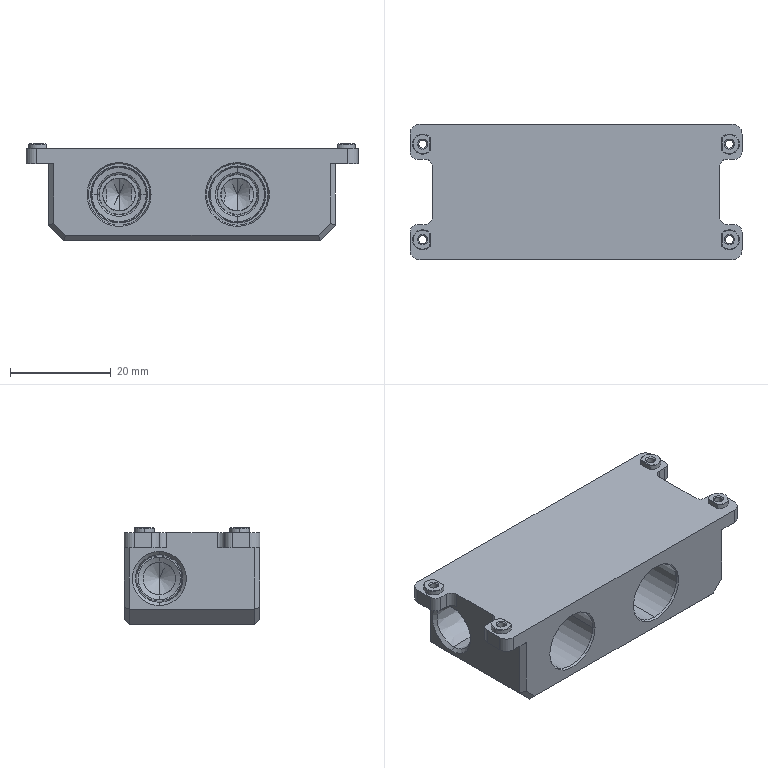NC program | NX | posted with a generic post | part box 66 x 27 x 19.25 mm
Lines 5135 to 6448 of 6448:
(CAVITY_MILL , TOOL : D3清角)
N10130 T04 M6
N10132 G54
N10134 G17 G0 G90 X-9.991 Y-7.014 S1061 M3
N10136 G43 Z20. H4
N10138 Z1.
N10140 G94 G1 X-10.477 Y-7.291 Z0.961 F250.
N10142 X-11.102 Y-8.064 Z0.891
N10144 X-11.353 Y-9.026 Z0.822
N10146 X-11.184 Y-10.006 Z0.752
N10148 X-10.625 Y-10.829 Z0.683
N10150 X-10.008 Y-11.254 Z0.63
N10152 X-9.386 Y-11.448 Z0.585
N10154 X-8.637 Y-11.452 Z0.532
N10156 X-7.699 Y-11.088 Z0.462
N10158 X-6.999 Y-10.366 Z0.392
N10160 X-6.71 Y-9.674 Z0.339
N10162 X-6.681 Y-8.712 Z0.272
N10164 X-7.04 Y-7.819 Z0.205
N10166 X-7.726 Y-7.144 Z0.137
N10168 X-8.625 Y-6.8 Z0.07
N10170 X-9.011 Z0.043
N10172 X-9.386 Y-6.802 Z0.017
N10174 X-9.826 Y-6.92 Z-0.015
N10176 X-10.477 Y-7.291 Z-0.067
N10178 X-11.102 Y-8.064 Z-0.137
N10180 X-11.353 Y-9.026 Z-0.206
N10182 X-11.184 Y-10.006 Z-0.276
N10184 X-10.625 Y-10.829 Z-0.346
N10186 X-10.008 Y-11.254 Z-0.398
N10188 X-9.386 Y-11.448 Z-0.443
N10190 X-8.637 Y-11.452 Z-0.496
N10192 X-7.699 Y-11.088 Z-0.566
N10194 X-6.999 Y-10.366 Z-0.637
N10196 X-6.71 Y-9.674 Z-0.689
N10198 X-6.681 Y-8.712 Z-0.756
N10200 X-7.04 Y-7.819 Z-0.824
N10202 X-7.726 Y-7.144 Z-0.891
N10204 X-8.625 Y-6.8 Z-0.958
N10206 X-9. Z-0.984
N10208 X-9.011
N10210 G3 X-11.325 Y-9.136 R2.325
N10212 X-9. Y-6.8 R-2.325
N10214 G1 Y-4.7
N10216 X-9.021
N10218 G3 X-13.425 Y-9.146 R4.425
N10220 X-9. Y-4.7 R-4.425
N10222 G1 Z0.016
N10224 G0 Z20.
N10226 X13.512 Y-7.037
N10228 Z1.
N10230 G1 X13.212 Y-7.154 Z0.977
N10232 X12.521 Y-7.848 Z0.909
N10234 X12.173 Y-8.764 Z0.84
N10236 X12.177 Y-9.514 Z0.788
N10238 X12.541 Y-10.432 Z0.719
N10240 X13.25 Y-11.121 Z0.65
N10242 X14.178 Y-11.458 Z0.581
N10244 X15.163 Y-11.385 Z0.512
N10246 X15.84 Y-11.062 Z0.459
N10248 X16.488 Y-10.387 Z0.394
N10250 X16.823 Y-9.514 Z0.328
N10252 X16.827 Y-8.764 Z0.276
N10254 X16.513 Y-7.903 Z0.212
N10256 X15.894 Y-7.227 Z0.148
N10258 X15.227 Y-6.885 Z0.095
N10260 X14.875 Y-6.8 Z0.07
N10262 X14.125 Z0.018
N10264 X13.212 Y-7.154 Z-0.051
N10266 X12.521 Y-7.848 Z-0.119
N10268 X12.173 Y-8.764 Z-0.188
N10270 X12.177 Y-9.514 Z-0.24
N10272 X12.541 Y-10.432 Z-0.309
N10274 X13.25 Y-11.121 Z-0.378
N10276 X14.178 Y-11.458 Z-0.447
N10278 X15.163 Y-11.385 Z-0.517
N10280 X15.84 Y-11.062 Z-0.569
N10282 X16.488 Y-10.387 Z-0.634
N10284 X16.823 Y-9.514 Z-0.7
N10286 X16.827 Y-8.764 Z-0.752
N10288 X16.513 Y-7.903 Z-0.816
N10290 X15.894 Y-7.227 Z-0.88
N10292 X15.227 Y-6.885 Z-0.933
N10294 X14.875 Y-6.8 Z-0.958
N10296 X14.5 Z-0.984
N10298 G3 X12.175 Y-9.125 R2.325
N10300 X14.5 Y-6.8 R-2.325
N10302 G1 Y-4.7
N10304 G3 X10.075 Y-9.125 R4.425
N10306 X14.5 Y-4.7 R-4.425
N10308 G1 Z0.016
N10310 G0 Z20.
N10312 X13.512 Y-7.037
N10314 Z0.016
N10316 G1 X13.212 Y-7.154 Z-0.007
N10318 X12.521 Y-7.848 Z-0.075
N10320 X12.173 Y-8.764 Z-0.144
N10322 X12.177 Y-9.514 Z-0.196
N10324 X12.541 Y-10.432 Z-0.265
N10326 X13.25 Y-11.121 Z-0.334
N10328 X14.178 Y-11.458 Z-0.404
N10330 X15.163 Y-11.385 Z-0.473
N10332 X15.84 Y-11.062 Z-0.525
N10334 X16.488 Y-10.387 Z-0.59
N10336 X16.823 Y-9.514 Z-0.656
N10338 X16.827 Y-8.764 Z-0.708
N10340 X16.513 Y-7.903 Z-0.772
N10342 X15.894 Y-7.227 Z-0.837
N10344 X15.227 Y-6.885 Z-0.889
N10346 X14.875 Y-6.8 Z-0.914
N10348 X14.125 Z-0.967
N10350 X13.212 Y-7.154 Z-1.035
N10352 X12.521 Y-7.848 Z-1.104
N10354 X12.173 Y-8.764 Z-1.172
N10356 X12.177 Y-9.514 Z-1.225
N10358 X12.541 Y-10.432 Z-1.294
N10360 X13.25 Y-11.121 Z-1.363
N10362 X14.178 Y-11.458 Z-1.432
N10364 X15.163 Y-11.385 Z-1.501
N10366 X15.84 Y-11.062 Z-1.553
N10368 X16.488 Y-10.387 Z-1.619
N10370 X16.823 Y-9.514 Z-1.684
N10372 X16.827 Y-8.764 Z-1.737
N10374 X16.513 Y-7.903 Z-1.801
N10376 X15.894 Y-7.227 Z-1.865
N10378 X15.227 Y-6.885 Z-1.917
N10380 X14.875 Y-6.8 Z-1.943
N10382 X14.5 Z-1.969
N10384 G3 X12.175 Y-9.125 R2.325
N10386 X14.5 Y-6.8 R-2.325
N10388 G1 Y-4.7
N10390 G3 X10.075 Y-9.125 R4.425
N10392 X14.5 Y-4.7 R-4.425
N10394 G1 Z-0.969
N10396 G0 Z20.
N10398 X-9.991 Y-7.014
N10400 Z0.016
N10402 G1 X-10.477 Y-7.291 Z-0.023
N10404 X-11.102 Y-8.064 Z-0.093
N10406 X-11.353 Y-9.026 Z-0.163
N10408 X-11.184 Y-10.006 Z-0.232
N10410 X-10.625 Y-10.829 Z-0.302
N10412 X-10.008 Y-11.254 Z-0.354
N10414 X-9.386 Y-11.448 Z-0.4
N10416 X-8.637 Y-11.452 Z-0.452
N10418 X-7.699 Y-11.088 Z-0.522
N10420 X-6.999 Y-10.366 Z-0.593
N10422 X-6.71 Y-9.674 Z-0.645
N10424 X-6.681 Y-8.712 Z-0.712
N10426 X-7.04 Y-7.819 Z-0.78
N10428 X-7.726 Y-7.144 Z-0.847
N10430 X-8.625 Y-6.8 Z-0.914
N10432 X-9.011 Z-0.941
N10434 X-9.386 Y-6.802 Z-0.967
N10436 X-9.826 Y-6.92 Z-0.999
N10438 X-10.477 Y-7.291 Z-1.052
N10440 X-11.102 Y-8.064 Z-1.121
N10442 X-11.353 Y-9.026 Z-1.191
N10444 X-11.184 Y-10.006 Z-1.26
N10446 X-10.625 Y-10.829 Z-1.33
N10448 X-10.008 Y-11.254 Z-1.382
N10450 X-9.386 Y-11.448 Z-1.428
N10452 X-8.637 Y-11.452 Z-1.48
N10454 X-7.699 Y-11.088 Z-1.551
N10456 X-6.999 Y-10.366 Z-1.621
N10458 X-6.71 Y-9.674 Z-1.673
N10460 X-6.681 Y-8.712 Z-1.741
N10462 X-7.04 Y-7.819 Z-1.808
N10464 X-7.726 Y-7.144 Z-1.875
N10466 X-8.625 Y-6.8 Z-1.943
N10468 X-9. Z-1.969
N10470 X-9.011
N10472 G3 X-11.325 Y-9.136 R2.325
N10474 X-9. Y-6.8 R-2.325
N10476 G1 Y-4.7
N10478 X-9.021
N10480 G3 X-13.425 Y-9.146 R4.425
N10482 X-9. Y-4.7 R-4.425
N10484 G1 Z-0.969
N10486 G0 Z20.
N10488 X-9.991 Y-7.014
N10490 Z-0.969
N10492 G1 X-10.477 Y-7.291 Z-1.008
N10494 X-11.102 Y-8.064 Z-1.077
N10496 X-11.353 Y-9.026 Z-1.147
N10498 X-11.184 Y-10.006 Z-1.216
N10500 X-10.625 Y-10.829 Z-1.286
N10502 X-10.008 Y-11.254 Z-1.338
N10504 X-9.386 Y-11.448 Z-1.384
N10506 X-8.637 Y-11.452 Z-1.436
N10508 X-7.699 Y-11.088 Z-1.507
N10510 X-6.999 Y-10.366 Z-1.577
N10512 X-6.71 Y-9.674 Z-1.629
N10514 X-6.681 Y-8.712 Z-1.697
N10516 X-7.04 Y-7.819 Z-1.764
N10518 X-7.726 Y-7.144 Z-1.831
N10520 X-8.625 Y-6.8 Z-1.899
N10522 X-9.011 Z-1.926
N10524 X-9.386 Y-6.802 Z-1.952
N10526 X-9.826 Y-6.92 Z-1.984
N10528 X-10.477 Y-7.291 Z-2.036
N10530 X-11.102 Y-8.064 Z-2.106
N10532 X-11.353 Y-9.026 Z-2.175
N10534 X-11.184 Y-10.006 Z-2.245
N10536 X-10.625 Y-10.829 Z-2.314
N10538 X-10.008 Y-11.254 Z-2.367
N10540 X-9.386 Y-11.448 Z-2.412
N10542 X-8.637 Y-11.452 Z-2.465
N10544 X-7.699 Y-11.088 Z-2.535
N10546 X-6.999 Y-10.366 Z-2.605
N10548 X-6.71 Y-9.674 Z-2.658
N10550 X-6.681 Y-8.712 Z-2.725
N10552 X-7.04 Y-7.819 Z-2.792
N10554 X-7.726 Y-7.144 Z-2.86
N10556 X-8.625 Y-6.8 Z-2.927
N10558 X-9. Z-2.953
N10560 X-9.011
N10562 G3 X-11.325 Y-9.136 R2.325
N10564 X-9. Y-6.8 R-2.325
N10566 G1 Y-4.7
N10568 X-9.021
N10570 G3 X-13.425 Y-9.146 R4.425
N10572 X-9. Y-4.7 R-4.425
N10574 G1 Z-1.953
N10576 G0 Z20.
N10578 X13.512 Y-7.037
N10580 Z-0.969
N10582 G1 X13.212 Y-7.154 Z-0.991
N10584 X12.521 Y-7.848 Z-1.06
N10586 X12.173 Y-8.764 Z-1.128
N10588 X12.177 Y-9.514 Z-1.181
N10590 X12.541 Y-10.432 Z-1.25
N10592 X13.25 Y-11.121 Z-1.319
N10594 X14.178 Y-11.458 Z-1.388
N10596 X15.163 Y-11.385 Z-1.457
N10598 X15.84 Y-11.062 Z-1.509
N10600 X16.488 Y-10.387 Z-1.575
N10602 X16.823 Y-9.514 Z-1.64
N10604 X16.827 Y-8.764 Z-1.693
N10606 X16.513 Y-7.903 Z-1.757
N10608 X15.894 Y-7.227 Z-1.821
N10610 X15.227 Y-6.885 Z-1.873
N10612 X14.875 Y-6.8 Z-1.899
N10614 X14.125 Z-1.951
N10616 X13.212 Y-7.154 Z-2.02
N10618 X12.521 Y-7.848 Z-2.088
N10620 X12.173 Y-8.764 Z-2.157
N10622 X12.177 Y-9.514 Z-2.209
N10624 X12.541 Y-10.432 Z-2.278
N10626 X13.25 Y-11.121 Z-2.347
N10628 X14.178 Y-11.458 Z-2.416
N10630 X15.163 Y-11.385 Z-2.485
N10632 X15.84 Y-11.062 Z-2.538
N10634 X16.488 Y-10.387 Z-2.603
N10636 X16.823 Y-9.514 Z-2.669
N10638 X16.827 Y-8.764 Z-2.721
N10640 X16.513 Y-7.903 Z-2.785
N10642 X15.894 Y-7.227 Z-2.849
N10644 X15.227 Y-6.885 Z-2.902
N10646 X14.875 Y-6.8 Z-2.927
N10648 X14.5 Z-2.953
N10650 G3 X12.175 Y-9.125 R2.325
N10652 X14.5 Y-6.8 R-2.325
N10654 G1 Y-4.7
N10656 G3 X10.075 Y-9.125 R4.425
N10658 X14.5 Y-4.7 R-4.425
N10660 G1 Z-1.953
N10662 G0 Z20.
N10664 X13.512 Y-7.037
N10666 Z-1.953
N10668 G1 X13.212 Y-7.154 Z-1.976
N10670 X12.521 Y-7.848 Z-2.044
N10672 X12.173 Y-8.764 Z-2.113
N10674 X12.177 Y-9.514 Z-2.165
N10676 X12.541 Y-10.432 Z-2.234
N10678 X13.25 Y-11.121 Z-2.303
N10680 X14.178 Y-11.458 Z-2.372
N10682 X15.163 Y-11.385 Z-2.441
N10684 X15.84 Y-11.062 Z-2.494
N10686 X16.488 Y-10.387 Z-2.559
N10688 X16.823 Y-9.514 Z-2.625
N10690 X16.827 Y-8.764 Z-2.677
N10692 X16.513 Y-7.903 Z-2.741
N10694 X15.894 Y-7.227 Z-2.805
N10696 X15.227 Y-6.885 Z-2.858
N10698 X14.875 Y-6.8 Z-2.883
N10700 X14.125 Z-2.935
N10702 X13.212 Y-7.154 Z-3.004
N10704 X12.521 Y-7.848 Z-3.072
N10706 X12.173 Y-8.764 Z-3.141
N10708 X12.177 Y-9.514 Z-3.193
N10710 X12.541 Y-10.432 Z-3.262
N10712 X13.25 Y-11.121 Z-3.332
N10714 X14.178 Y-11.458 Z-3.401
N10716 X15.163 Y-11.385 Z-3.47
N10718 X15.84 Y-11.062 Z-3.522
N10720 X16.488 Y-10.387 Z-3.588
N10722 X16.823 Y-9.514 Z-3.653
N10724 X16.827 Y-8.764 Z-3.705
N10726 X16.513 Y-7.903 Z-3.769
N10728 X15.894 Y-7.227 Z-3.834
N10730 X15.227 Y-6.885 Z-3.886
N10732 X14.875 Y-6.8 Z-3.911
N10734 X14.5 Z-3.938
N10736 G3 X12.175 Y-9.125 R2.325
N10738 X14.5 Y-6.8 R-2.325
N10740 G1 Y-4.7
N10742 G3 X10.075 Y-9.125 R4.425
N10744 X14.5 Y-4.7 R-4.425
N10746 G1 Z-2.938
N10748 G0 Z20.
N10750 X-9.991 Y-7.014
N10752 Z-1.953
N10754 G1 X-10.477 Y-7.291 Z-1.992
N10756 X-11.102 Y-8.064 Z-2.062
N10758 X-11.353 Y-9.026 Z-2.131
N10760 X-11.184 Y-10.006 Z-2.201
N10762 X-10.625 Y-10.829 Z-2.27
N10764 X-10.008 Y-11.254 Z-2.323
N10766 X-9.386 Y-11.448 Z-2.368
N10768 X-8.637 Y-11.452 Z-2.421
N10770 X-7.699 Y-11.088 Z-2.491
N10772 X-6.999 Y-10.366 Z-2.561
N10774 X-6.71 Y-9.674 Z-2.614
N10776 X-6.681 Y-8.712 Z-2.681
N10778 X-7.04 Y-7.819 Z-2.748
N10780 X-7.726 Y-7.144 Z-2.816
N10782 X-8.625 Y-6.8 Z-2.883
N10784 X-9.011 Z-2.91
N10786 X-9.386 Y-6.802 Z-2.936
N10788 X-9.826 Y-6.92 Z-2.968
N10790 X-10.477 Y-7.291 Z-3.02
N10792 X-11.102 Y-8.064 Z-3.09
N10794 X-11.353 Y-9.026 Z-3.16
N10796 X-11.184 Y-10.006 Z-3.229
N10798 X-10.625 Y-10.829 Z-3.299
N10800 X-10.008 Y-11.254 Z-3.351
N10802 X-9.386 Y-11.448 Z-3.397
N10804 X-8.637 Y-11.452 Z-3.449
N10806 X-7.699 Y-11.088 Z-3.519
N10808 X-6.999 Y-10.366 Z-3.59
N10810 X-6.71 Y-9.674 Z-3.642
N10812 X-6.681 Y-8.712 Z-3.709
N10814 X-7.04 Y-7.819 Z-3.777
N10816 X-7.726 Y-7.144 Z-3.844
N10818 X-8.625 Y-6.8 Z-3.911
N10820 X-9. Z-3.938
N10822 X-9.011
N10824 G3 X-11.325 Y-9.136 R2.325
N10826 X-9. Y-6.8 R-2.325
N10828 G1 Y-4.7
N10830 X-9.021
N10832 G3 X-13.425 Y-9.146 R4.425
N10834 X-9. Y-4.7 R-4.425
N10836 G1 Z-2.938
N10838 G0 Z20.
N10840 X-9.991 Y-7.014
N10842 Z-2.938
N10844 G1 X-10.477 Y-7.291 Z-2.977
N10846 X-11.102 Y-8.064 Z-3.046
N10848 X-11.353 Y-9.026 Z-3.116
N10850 X-11.184 Y-10.006 Z-3.185
N10852 X-10.625 Y-10.829 Z-3.255
N10854 X-10.008 Y-11.254 Z-3.307
N10856 X-9.386 Y-11.448 Z-3.353
N10858 X-8.637 Y-11.452 Z-3.405
N10860 X-7.699 Y-11.088 Z-3.475
N10862 X-6.999 Y-10.366 Z-3.546
N10864 X-6.71 Y-9.674 Z-3.598
N10866 X-6.681 Y-8.712 Z-3.665
N10868 X-7.04 Y-7.819 Z-3.733
N10870 X-7.726 Y-7.144 Z-3.8
N10872 X-8.625 Y-6.8 Z-3.867
N10874 X-9.011 Z-3.894
N10876 X-9.386 Y-6.802 Z-3.921
N10878 X-9.826 Y-6.92 Z-3.952
N10880 X-10.477 Y-7.291 Z-4.005
N10882 X-11.102 Y-8.064 Z-4.074
N10884 X-11.353 Y-9.026 Z-4.144
N10886 X-11.184 Y-10.006 Z-4.213
N10888 X-10.625 Y-10.829 Z-4.283
N10890 X-10.008 Y-11.254 Z-4.335
N10892 X-9.386 Y-11.448 Z-4.381
N10894 X-8.637 Y-11.452 Z-4.433
N10896 X-7.699 Y-11.088 Z-4.504
N10898 X-6.999 Y-10.366 Z-4.574
N10900 X-6.71 Y-9.674 Z-4.626
N10902 X-6.681 Y-8.712 Z-4.694
N10904 X-7.04 Y-7.819 Z-4.761
N10906 X-7.726 Y-7.144 Z-4.828
N10908 X-8.625 Y-6.8 Z-4.896
N10910 X-9. Z-4.922
N10912 X-9.011
N10914 G3 X-11.325 Y-9.136 R2.325
N10916 X-9. Y-6.8 R-2.325
N10918 G1 Y-4.7
N10920 X-9.021
N10922 G3 X-13.425 Y-9.146 R4.425
N10924 X-9. Y-4.7 R-4.425
N10926 G1 Z-3.922
N10928 G0 Z20.
N10930 X13.512 Y-7.037
N10932 Z-2.938
N10934 G1 X13.212 Y-7.154 Z-2.96
N10936 X12.521 Y-7.848 Z-3.029
N10938 X12.173 Y-8.764 Z-3.097
N10940 X12.177 Y-9.514 Z-3.149
N10942 X12.541 Y-10.432 Z-3.219
N10944 X13.25 Y-11.121 Z-3.288
N10946 X14.178 Y-11.458 Z-3.357
N10948 X15.163 Y-11.385 Z-3.426
N10950 X15.84 Y-11.062 Z-3.478
N10952 X16.488 Y-10.387 Z-3.544
N10954 X16.823 Y-9.514 Z-3.609
N10956 X16.827 Y-8.764 Z-3.661
N10958 X16.513 Y-7.903 Z-3.726
N10960 X15.894 Y-7.227 Z-3.79
N10962 X15.227 Y-6.885 Z-3.842
N10964 X14.875 Y-6.8 Z-3.867
N10966 X14.125 Z-3.92
N10968 X13.212 Y-7.154 Z-3.988
N10970 X12.521 Y-7.848 Z-4.057
N10972 X12.173 Y-8.764 Z-4.125
N10974 X12.177 Y-9.514 Z-4.178
N10976 X12.541 Y-10.432 Z-4.247
N10978 X13.25 Y-11.121 Z-4.316
N10980 X14.178 Y-11.458 Z-4.385
N10982 X15.163 Y-11.385 Z-4.454
N10984 X15.84 Y-11.062 Z-4.506
N10986 X16.488 Y-10.387 Z-4.572
N10988 X16.823 Y-9.514 Z-4.637
N10990 X16.827 Y-8.764 Z-4.69
N10992 X16.513 Y-7.903 Z-4.754
N10994 X15.894 Y-7.227 Z-4.818
N10996 X15.227 Y-6.885 Z-4.87
N10998 X14.875 Y-6.8 Z-4.896
N11000 X14.5 Z-4.922
N11002 G3 X12.175 Y-9.125 R2.325
N11004 X14.5 Y-6.8 R-2.325
N11006 G1 Y-4.7
N11008 G3 X10.075 Y-9.125 R4.425
N11010 X14.5 Y-4.7 R-4.425
N11012 G1 Z-3.922
N11014 G0 Z20.
N11016 X13.512 Y-7.037
N11018 Z-3.922
N11020 G1 X13.212 Y-7.154 Z-3.944
N11022 X12.521 Y-7.848 Z-4.013
N11024 X12.173 Y-8.764 Z-4.081
N11026 X12.177 Y-9.514 Z-4.134
N11028 X12.541 Y-10.432 Z-4.203
N11030 X13.25 Y-11.121 Z-4.272
N11032 X14.178 Y-11.458 Z-4.341
N11034 X15.163 Y-11.385 Z-4.41
N11036 X15.84 Y-11.062 Z-4.463
N11038 X16.488 Y-10.387 Z-4.528
N11040 X16.823 Y-9.514 Z-4.593
N11042 X16.827 Y-8.764 Z-4.646
N11044 X16.513 Y-7.903 Z-4.71
N11046 X15.894 Y-7.227 Z-4.774
N11048 X15.227 Y-6.885 Z-4.826
N11050 X14.875 Y-6.8 Z-4.852
N11052 X14.125 Z-4.904
N11054 X13.212 Y-7.154 Z-4.973
N11056 X12.521 Y-7.848 Z-5.041
N11058 X12.173 Y-8.764 Z-5.11
N11060 X12.177 Y-9.514 Z-5.162
N11062 X12.541 Y-10.432 Z-5.231
N11064 X13.25 Y-11.121 Z-5.3
N11066 X14.178 Y-11.458 Z-5.369
N11068 X15.163 Y-11.385 Z-5.438
N11070 X15.84 Y-11.062 Z-5.491
N11072 X16.488 Y-10.387 Z-5.556
N11074 X16.823 Y-9.514 Z-5.622
N11076 X16.827 Y-8.764 Z-5.674
N11078 X16.513 Y-7.903 Z-5.738
N11080 X15.894 Y-7.227 Z-5.802
N11082 X15.227 Y-6.885 Z-5.855
N11084 X14.875 Y-6.8 Z-5.88
N11086 X14.5 Z-5.906
N11088 G3 X12.175 Y-9.125 R2.325
N11090 X14.5 Y-6.8 R-2.325
N11092 G1 Y-4.7
N11094 G3 X10.075 Y-9.125 R4.425
N11096 X14.5 Y-4.7 R-4.425
N11098 G1 Z-4.906
N11100 G0 Z20.
N11102 X-9.991 Y-7.014
N11104 Z-3.922
N11106 G1 X-10.477 Y-7.291 Z-3.961
N11108 X-11.102 Y-8.064 Z-4.031
N11110 X-11.353 Y-9.026 Z-4.1
N11112 X-11.184 Y-10.006 Z-4.17
N11114 X-10.625 Y-10.829 Z-4.239
N11116 X-10.008 Y-11.254 Z-4.292
N11118 X-9.386 Y-11.448 Z-4.337
N11120 X-8.637 Y-11.452 Z-4.389
N11122 X-7.699 Y-11.088 Z-4.46
N11124 X-6.999 Y-10.366 Z-4.53
N11126 X-6.71 Y-9.674 Z-4.583
N11128 X-6.681 Y-8.712 Z-4.65
N11130 X-7.04 Y-7.819 Z-4.717
N11132 X-7.726 Y-7.144 Z-4.784
N11134 X-8.625 Y-6.8 Z-4.852
N11136 X-9.011 Z-4.879
N11138 X-9.386 Y-6.802 Z-4.905
N11140 X-9.826 Y-6.92 Z-4.937
N11142 X-10.477 Y-7.291 Z-4.989
N11144 X-11.102 Y-8.064 Z-5.059
N11146 X-11.353 Y-9.026 Z-5.128
N11148 X-11.184 Y-10.006 Z-5.198
N11150 X-10.625 Y-10.829 Z-5.267
N11152 X-10.008 Y-11.254 Z-5.32
N11154 X-9.386 Y-11.448 Z-5.365
N11156 X-8.637 Y-11.452 Z-5.418
N11158 X-7.699 Y-11.088 Z-5.488
N11160 X-6.999 Y-10.366 Z-5.558
N11162 X-6.71 Y-9.674 Z-5.611
N11164 X-6.681 Y-8.712 Z-5.678
N11166 X-7.04 Y-7.819 Z-5.745
N11168 X-7.726 Y-7.144 Z-5.813
N11170 X-8.625 Y-6.8 Z-5.88
N11172 X-9. Z-5.906
N11174 X-9.011
N11176 G3 X-11.325 Y-9.136 R2.325
N11178 X-9. Y-6.8 R-2.325
N11180 G1 Y-4.7
N11182 X-9.021
N11184 G3 X-13.425 Y-9.146 R4.425
N11186 X-9. Y-4.7 R-4.425
N11188 G1 Z-4.906
N11190 G0 Z20.
N11192 X-9.991 Y-7.014
N11194 Z-4.906
N11196 G1 X-10.477 Y-7.291 Z-4.945
N11198 X-11.102 Y-8.064 Z-5.015
N11200 X-11.353 Y-9.026 Z-5.084
N11202 X-11.184 Y-10.006 Z-5.154
N11204 X-10.625 Y-10.829 Z-5.224
N11206 X-10.008 Y-11.254 Z-5.276
N11208 X-9.386 Y-11.448 Z-5.321
N11210 X-8.637 Y-11.452 Z-5.374
N11212 X-7.699 Y-11.088 Z-5.444
N11214 X-6.999 Y-10.366 Z-5.515
N11216 X-6.71 Y-9.674 Z-5.567
N11218 X-6.681 Y-8.712 Z-5.634
N11220 X-7.04 Y-7.819 Z-5.702
N11222 X-7.726 Y-7.144 Z-5.769
N11224 X-8.625 Y-6.8 Z-5.836
N11226 X-9.011 Z-5.863
N11228 X-9.386 Y-6.802 Z-5.889
N11230 X-9.826 Y-6.92 Z-5.921
N11232 X-10.477 Y-7.291 Z-5.974
N11234 X-11.102 Y-8.064 Z-6.043
N11236 X-11.353 Y-9.026 Z-6.113
N11238 X-11.184 Y-10.006 Z-6.182
N11240 X-10.625 Y-10.829 Z-6.252
N11242 X-10.008 Y-11.254 Z-6.304
N11244 X-9.386 Y-11.448 Z-6.35
N11246 X-8.637 Y-11.452 Z-6.402
N11248 X-7.699 Y-11.088 Z-6.472
N11250 X-6.999 Y-10.366 Z-6.543
N11252 X-6.71 Y-9.674 Z-6.595
N11254 X-6.681 Y-8.712 Z-6.663
N11256 X-7.04 Y-7.819 Z-6.73
N11258 X-7.726 Y-7.144 Z-6.797
N11260 X-8.625 Y-6.8 Z-6.864
N11262 X-9. Z-6.891
N11264 X-9.011
N11266 G3 X-11.325 Y-9.136 R2.325
N11268 X-9. Y-6.8 R-2.325
N11270 G1 Y-4.7
N11272 X-9.021
N11274 G3 X-13.425 Y-9.146 R4.425
N11276 X-9. Y-4.7 R-4.425
N11278 G1 Z-5.891
N11280 G0 Z20.
N11282 X13.512 Y-7.037
N11284 Z-4.906
N11286 G1 X13.212 Y-7.154 Z-4.929
N11288 X12.521 Y-7.848 Z-4.997
N11290 X12.173 Y-8.764 Z-5.066
N11292 X12.177 Y-9.514 Z-5.118
N11294 X12.541 Y-10.432 Z-5.187
N11296 X13.25 Y-11.121 Z-5.256
N11298 X14.178 Y-11.458 Z-5.325
N11300 X15.163 Y-11.385 Z-5.395
N11302 X15.84 Y-11.062 Z-5.447
N11304 X16.488 Y-10.387 Z-5.512
N11306 X16.823 Y-9.514 Z-5.578
N11308 X16.827 Y-8.764 Z-5.63
N11310 X16.513 Y-7.903 Z-5.694
N11312 X15.894 Y-7.227 Z-5.758
N11314 X15.227 Y-6.885 Z-5.811
N11316 X14.875 Y-6.8 Z-5.836
N11318 X14.125 Z-5.889
N11320 X13.212 Y-7.154 Z-5.957
N11322 X12.521 Y-7.848 Z-6.026
N11324 X12.173 Y-8.764 Z-6.094
N11326 X12.177 Y-9.514 Z-6.146
N11328 X12.541 Y-10.432 Z-6.216
N11330 X13.25 Y-11.121 Z-6.285
N11332 X14.178 Y-11.458 Z-6.354
N11334 X15.163 Y-11.385 Z-6.423
N11336 X15.84 Y-11.062 Z-6.475
N11338 X16.488 Y-10.387 Z-6.541
N11340 X16.823 Y-9.514 Z-6.606
N11342 X16.827 Y-8.764 Z-6.658
N11344 X16.513 Y-7.903 Z-6.723
N11346 X15.894 Y-7.227 Z-6.787
N11348 X15.227 Y-6.885 Z-6.839
N11350 X14.875 Y-6.8 Z-6.864
N11352 X14.5 Z-6.891
N11354 G3 X12.175 Y-9.125 R2.325
N11356 X14.5 Y-6.8 R-2.325
N11358 G1 Y-4.7
N11360 G3 X10.075 Y-9.125 R4.425
N11362 X14.5 Y-4.7 R-4.425
N11364 G1 Z-5.891
N11366 G0 Z20.
N11368 X13.512 Y-7.037
N11370 Z-5.891
N11372 G1 X13.212 Y-7.154 Z-5.913
N11374 X12.521 Y-7.848 Z-5.982
N11376 X12.173 Y-8.764 Z-6.05
N11378 X12.177 Y-9.514 Z-6.103
N11380 X12.541 Y-10.432 Z-6.172
N11382 X13.25 Y-11.121 Z-6.241
N11384 X14.178 Y-11.458 Z-6.31
N11386 X15.163 Y-11.385 Z-6.379
N11388 X15.84 Y-11.062 Z-6.431
N11390 X16.488 Y-10.387 Z-6.497
N11392 X16.823 Y-9.514 Z-6.562
N11394 X16.827 Y-8.764 Z-6.615
N11396 X16.513 Y-7.903 Z-6.679
N11398 X15.894 Y-7.227 Z-6.743
N11400 X15.227 Y-6.885 Z-6.795
N11402 X14.875 Y-6.8 Z-6.821
N11404 X14.125 Z-6.873
N11406 X13.212 Y-7.154 Z-6.941
N11408 X12.521 Y-7.848 Z-7.01
N11410 X12.173 Y-8.764 Z-7.078
N11412 X12.177 Y-9.514 Z-7.131
N11414 X12.541 Y-10.432 Z-7.2
N11416 X13.25 Y-11.121 Z-7.269
N11418 X14.178 Y-11.458 Z-7.338
N11420 X15.163 Y-11.385 Z-7.407
N11422 X15.84 Y-11.062 Z-7.46
N11424 X16.488 Y-10.387 Z-7.525
N11426 X16.823 Y-9.514 Z-7.59
N11428 X16.827 Y-8.764 Z-7.643
N11430 X16.513 Y-7.903 Z-7.707
N11432 X15.894 Y-7.227 Z-7.771
N11434 X15.227 Y-6.885 Z-7.823
N11436 X14.875 Y-6.8 Z-7.849
N11438 X14.5 Z-7.875
N11440 G3 X12.175 Y-9.125 R2.325
N11442 X14.5 Y-6.8 R-2.325
N11444 G1 Y-4.7
N11446 G3 X10.075 Y-9.125 R4.425
N11448 X14.5 Y-4.7 R-4.425
N11450 G1 Z-6.875
N11452 G0 Z20.
N11454 X-9.991 Y-7.014
N11456 Z-5.891
N11458 G1 X-10.477 Y-7.291 Z-5.93
N11460 X-11.102 Y-8.064 Z-5.999
N11462 X-11.353 Y-9.026 Z-6.069
N11464 X-11.184 Y-10.006 Z-6.138
N11466 X-10.625 Y-10.829 Z-6.208
N11468 X-10.008 Y-11.254 Z-6.26
N11470 X-9.386 Y-11.448 Z-6.306
N11472 X-8.637 Y-11.452 Z-6.358
N11474 X-7.699 Y-11.088 Z-6.429
N11476 X-6.999 Y-10.366 Z-6.499
N11478 X-6.71 Y-9.674 Z-6.551
N11480 X-6.681 Y-8.712 Z-6.619
N11482 X-7.04 Y-7.819 Z-6.686
N11484 X-7.726 Y-7.144 Z-6.753
N11486 X-8.625 Y-6.8 Z-6.821
N11488 X-9.011 Z-6.848
N11490 X-9.386 Y-6.802 Z-6.874
N11492 X-9.826 Y-6.92 Z-6.906
N11494 X-10.477 Y-7.291 Z-6.958
N11496 X-11.102 Y-8.064 Z-7.028
N11498 X-11.353 Y-9.026 Z-7.097
N11500 X-11.184 Y-10.006 Z-7.167
N11502 X-10.625 Y-10.829 Z-7.236
N11504 X-10.008 Y-11.254 Z-7.289
N11506 X-9.386 Y-11.448 Z-7.334
N11508 X-8.637 Y-11.452 Z-7.387
N11510 X-7.699 Y-11.088 Z-7.457
N11512 X-6.999 Y-10.366 Z-7.527
N11514 X-6.71 Y-9.674 Z-7.58
N11516 X-6.681 Y-8.712 Z-7.647
N11518 X-7.04 Y-7.819 Z-7.714
N11520 X-7.726 Y-7.144 Z-7.781
N11522 X-8.625 Y-6.8 Z-7.849
N11524 X-9. Z-7.875
N11526 X-9.011
N11528 G3 X-11.325 Y-9.136 R2.325
N11530 X-9. Y-6.8 R-2.325
N11532 G1 Y-4.7
N11534 X-9.021
N11536 G3 X-13.425 Y-9.146 R4.425
N11538 X-9. Y-4.7 R-4.425
N11540 G1 Z-6.875
N11542 G0 Z20.
N11544 X-9.991 Y-7.014
N11546 Z-6.875
N11548 G1 X-10.477 Y-7.291 Z-6.914
N11550 X-11.102 Y-8.064 Z-6.984
N11552 X-11.353 Y-9.026 Z-7.053
N11554 X-11.184 Y-10.006 Z-7.123
N11556 X-10.625 Y-10.829 Z-7.192
N11558 X-10.008 Y-11.254 Z-7.245
N11560 X-9.386 Y-11.448 Z-7.29
N11562 X-8.637 Y-11.452 Z-7.343
N11564 X-7.699 Y-11.088 Z-7.413
N11566 X-6.999 Y-10.366 Z-7.483
N11568 X-6.71 Y-9.674 Z-7.536
N11570 X-6.681 Y-8.712 Z-7.603
N11572 X-7.04 Y-7.819 Z-7.67
N11574 X-7.726 Y-7.144 Z-7.738
N11576 X-8.625 Y-6.8 Z-7.805
N11578 X-9.011 Z-7.832
N11580 X-9.386 Y-6.802 Z-7.858
N11582 X-9.826 Y-6.92 Z-7.89
N11584 X-10.477 Y-7.291 Z-7.942
N11586 X-11.102 Y-8.064 Z-8.012
N11588 X-11.353 Y-9.026 Z-8.081
N11590 X-11.184 Y-10.006 Z-8.151
N11592 X-10.625 Y-10.829 Z-8.221
N11594 X-10.008 Y-11.254 Z-8.273
N11596 X-9.386 Y-11.448 Z-8.318
N11598 X-8.637 Y-11.452 Z-8.371
N11600 X-7.699 Y-11.088 Z-8.441
N11602 X-6.999 Y-10.366 Z-8.512
N11604 X-6.71 Y-9.674 Z-8.564
N11606 X-6.681 Y-8.712 Z-8.631
N11608 X-7.04 Y-7.819 Z-8.699
N11610 X-7.726 Y-7.144 Z-8.766
N11612 X-8.625 Y-6.8 Z-8.833
N11614 X-9. Z-8.859
N11616 X-9.011
N11618 G3 X-11.325 Y-9.136 R2.325
N11620 X-9. Y-6.8 R-2.325
N11622 G1 Y-4.7
N11624 X-9.021
N11626 G3 X-13.425 Y-9.146 R4.425
N11628 X-9. Y-4.7 R-4.425
N11630 G1 Z-7.859
N11632 G0 Z20.
N11634 X13.512 Y-7.037
N11636 Z-6.875
N11638 G1 X13.212 Y-7.154 Z-6.898
N11640 X12.521 Y-7.848 Z-6.966
N11642 X12.173 Y-8.764 Z-7.035
N11644 X12.177 Y-9.514 Z-7.087
N11646 X12.541 Y-10.432 Z-7.156
N11648 X13.25 Y-11.121 Z-7.225
N11650 X14.178 Y-11.458 Z-7.294
N11652 X15.163 Y-11.385 Z-7.363
N11654 X15.84 Y-11.062 Z-7.416
N11656 X16.488 Y-10.387 Z-7.481
N11658 X16.823 Y-9.514 Z-7.547
N11660 X16.827 Y-8.764 Z-7.599
N11662 X16.513 Y-7.903 Z-7.663
N11664 X15.894 Y-7.227 Z-7.727
N11666 X15.227 Y-6.885 Z-7.78
N11668 X14.875 Y-6.8 Z-7.805
N11670 X14.125 Z-7.857
N11672 X13.212 Y-7.154 Z-7.926
N11674 X12.521 Y-7.848 Z-7.994
N11676 X12.173 Y-8.764 Z-8.063
N11678 X12.177 Y-9.514 Z-8.115
N11680 X12.541 Y-10.432 Z-8.184
N11682 X13.25 Y-11.121 Z-8.253
N11684 X14.178 Y-11.458 Z-8.322
N11686 X15.163 Y-11.385 Z-8.392
N11688 X15.84 Y-11.062 Z-8.444
N11690 X16.488 Y-10.387 Z-8.509
N11692 X16.823 Y-9.514 Z-8.575
N11694 X16.827 Y-8.764 Z-8.627
N11696 X16.513 Y-7.903 Z-8.691
N11698 X15.894 Y-7.227 Z-8.755
N11700 X15.227 Y-6.885 Z-8.808
N11702 X14.875 Y-6.8 Z-8.833
N11704 X14.5 Z-8.859
N11706 G3 X12.175 Y-9.125 R2.325
N11708 X14.5 Y-6.8 R-2.325
N11710 G1 Y-4.7
N11712 G3 X10.075 Y-9.125 R4.425
N11714 X14.5 Y-4.7 R-4.425
N11716 G1 Z-7.859
N11718 G0 Z20.
N11720 X12.599 Y-7.641
N11722 Z-7.859
N11724 G1 X12.44 Y-7.801 Z-7.875
N11726 X12.079 Y-8.759 Z-7.947
N11728 X12.084 Y-9.523 Z-8.
N11730 X12.483 Y-10.514 Z-8.075
N11732 X13.266 Y-11.24 Z-8.15
N11734 X14.284 Y-11.564 Z-8.224
N11736 X15.343 Y-11.424 Z-8.299
N11738 X16.01 Y-11.053 Z-8.352
N11740 X16.615 Y-10.359 Z-8.417
N11742 X16.921 Y-9.491 Z-8.481
N11744 X16.916 Y-8.727 Z-8.535
N11746 X16.607 Y-7.877 Z-8.598
N11748 X16.01 Y-7.197 Z-8.661
N11750 X15.343 Y-6.826 Z-8.714
N11752 X14.882 Y-6.706 Z-8.748
N11754 X14.118 Z-8.801
N11756 X13.162 Y-7.074 Z-8.873
N11758 X12.44 Y-7.801 Z-8.944
N11760 X12.079 Y-8.759 Z-9.016
N11762 X12.084 Y-9.523 Z-9.07
N11764 X12.483 Y-10.514 Z-9.144
N11766 X13.266 Y-11.24 Z-9.219
N11768 X14.284 Y-11.564 Z-9.294
N11770 X15.343 Y-11.424 Z-9.368
N11772 X16.01 Y-11.053 Z-9.422
N11774 X16.615 Y-10.359 Z-9.486
N11776 X16.921 Y-9.491 Z-9.55
N11778 X16.916 Y-8.727 Z-9.604
N11780 X16.607 Y-7.877 Z-9.667
N11782 X16.01 Y-7.197 Z-9.73
N11784 X15.343 Y-6.826 Z-9.784
N11786 X14.882 Y-6.706 Z-9.817
N11788 X14.5 Z-9.844
N11790 G3 X12.081 Y-9.125 R2.419
N11792 X14.5 Y-6.706 R-2.419
N11794 G1 Y-5.206
N11796 G3 X10.581 Y-9.125 R3.919
N11798 X14.5 Y-5.206 R-3.919
N11800 G1 Z-8.844
N11802 G0 Z20.
N11804 X-10.895 Y-7.657
N11806 Z-7.859
N11808 G1 X-11.261 Y-8.185 Z-7.904
N11810 X-11.448 Y-9.205 Z-7.977
N11812 X-11.195 Y-10.21 Z-8.049
N11814 X-10.55 Y-11.021 Z-8.122
N11816 X-9.89 Y-11.407 Z-8.175
N11818 X-9.395 Y-11.542 Z-8.211
N11820 X-8.63 Y-11.546 Z-8.265
N11822 X-7.931 Y-11.328 Z-8.316
N11824 X-7.327 Y-10.913 Z-8.367
N11826 X-6.873 Y-10.338 Z-8.418
N11828 X-6.602 Y-9.623 Z-8.472
N11830 X-6.6 Y-8.639 Z-8.541
N11832 X-6.985 Y-7.733 Z-8.609
N11834 X-7.696 Y-7.052 Z-8.678
N11836 X-8.618 Y-6.706 Z-8.747
N11838 X-9.012 Z-8.775
N11840 X-9.395 Y-6.708 Z-8.801
N11842 X-10.036 Y-6.906 Z-8.848
N11844 X-10.67 Y-7.334 Z-8.902
N11846 X-11.261 Y-8.185 Z-8.974
N11848 X-11.448 Y-9.205 Z-9.047
N11850 X-11.195 Y-10.21 Z-9.119
N11852 X-10.55 Y-11.021 Z-9.192
N11854 X-9.89 Y-11.407 Z-9.245
N11856 X-9.395 Y-11.542 Z-9.281
N11858 X-8.63 Y-11.546 Z-9.335
N11860 X-7.931 Y-11.328 Z-9.386
N11862 X-7.327 Y-10.913 Z-9.437
N11864 X-6.873 Y-10.338 Z-9.488
N11866 X-6.602 Y-9.623 Z-9.542
N11868 X-6.6 Y-8.639 Z-9.611
N11870 X-6.985 Y-7.733 Z-9.679
N11872 X-7.696 Y-7.052 Z-9.748
N11874 X-8.618 Y-6.706 Z-9.817
N11876 X-9. Z-9.844
N11878 X-9.012
N11880 G3 X-11.419 Y-9.137 R2.419
N11882 X-9. Y-6.706 R-2.419
N11884 G1 Y-5.206
N11886 X-9.02
N11888 G3 X-12.919 Y-9.145 R3.919
N11890 X-9. Y-5.206 R-3.919
N11892 G1 Z-8.844
N11894 G0 Z20.
N11896 X-10.514 Y-7.311
N11898 Z-8.844
N11900 G1 X-11.023 Y-7.824 Z-8.894
N11902 X-11.377 Y-8.757 Z-8.964
N11904 X-11.373 Y-9.514 Z-9.017
N11906 X-11.015 Y-10.438 Z-9.086
N11908 X-10.315 Y-11.139 Z-9.156
N11910 X-9.392 Y-11.498 Z-9.225
N11912 X-8.634 Y-11.502 Z-9.278
N11914 X-7.927 Y-11.277 Z-9.33
N11916 X-7.322 Y-10.848 Z-9.382
N11918 X-6.876 Y-10.254 Z-9.433
N11920 X-6.631 Y-9.537 Z-9.486
N11922 X-6.655 Y-8.591 Z-9.553
N11924 X-7.043 Y-7.727 Z-9.619
N11926 X-7.734 Y-7.08 Z-9.685
N11928 X-8.621 Y-6.75 Z-9.751
N11930 X-9.013 Z-9.779
N11932 X-9.392 Y-6.752 Z-9.805
N11934 X-10.321 Y-7.115 Z-9.875
N11936 X-11.023 Y-7.824 Z-9.945
N11938 X-11.377 Y-8.757 Z-10.014
N11940 X-11.373 Y-9.514 Z-10.067
N11942 X-11.015 Y-10.438 Z-10.137
N11944 X-10.315 Y-11.139 Z-10.206
N11946 X-9.392 Y-11.498 Z-10.275
N11948 X-8.634 Y-11.502 Z-10.328
N11950 X-7.927 Y-11.277 Z-10.38
N11952 X-7.322 Y-10.848 Z-10.432
N11954 X-6.876 Y-10.254 Z-10.484
N11956 X-6.631 Y-9.537 Z-10.537
N11958 X-6.655 Y-8.591 Z-10.603
N11960 X-7.043 Y-7.727 Z-10.669
N11962 X-7.734 Y-7.08 Z-10.735
N11964 X-8.621 Y-6.75 Z-10.802
N11966 X-9. Z-10.828
N11968 X-9.013
N11970 G3 X-11.375 Y-9.138 R2.375
N11972 X-9. Y-6.75 R-2.375
N11974 G1 Y-5.25
N11976 X-9.021
N11978 G3 X-12.875 Y-9.146 R3.875
N11980 X-9. Y-5.25 R-3.875
N11982 G1 Z-9.828
N11984 G0 Z20.
N11986 X12.991 Y-7.307
N11988 Z-8.844
N11990 G1 X12.478 Y-7.824 Z-8.895
N11992 X12.122 Y-8.763 Z-8.965
N11994 X12.128 Y-9.52 Z-9.018
N11996 X12.522 Y-10.494 Z-9.091
N11998 X13.295 Y-11.206 Z-9.165
N12000 X14.297 Y-11.521 Z-9.238
N12002 X15.339 Y-11.379 Z-9.312
N12004 X15.998 Y-11.007 Z-9.365
N12006 X16.573 Y-10.344 Z-9.426
N12008 X16.872 Y-9.52 Z-9.487
N12010 X16.878 Y-8.763 Z-9.54
N12012 X16.581 Y-7.92 Z-9.603
N12014 X15.998 Y-7.243 Z-9.665
N12016 X15.339 Y-6.871 Z-9.718
N12018 X14.879 Y-6.75 Z-9.752
N12020 X14.121 Z-9.804
N12022 X13.185 Y-7.111 Z-9.875
N12024 X12.478 Y-7.824 Z-9.945
N12026 X12.122 Y-8.763 Z-10.015
N12028 X12.128 Y-9.52 Z-10.068
N12030 X12.522 Y-10.494 Z-10.141
N12032 X13.295 Y-11.206 Z-10.215
N12034 X14.297 Y-11.521 Z-10.288
N12036 X15.339 Y-11.379 Z-10.362
N12038 X15.998 Y-11.007 Z-10.415
N12040 X16.573 Y-10.344 Z-10.476
N12042 X16.872 Y-9.52 Z-10.538
N12044 X16.878 Y-8.763 Z-10.591
N12046 X16.581 Y-7.92 Z-10.653
N12048 X15.998 Y-7.243 Z-10.715
N12050 X15.339 Y-6.871 Z-10.768
N12052 X14.879 Y-6.75 Z-10.802
N12054 X14.5 Z-10.828
N12056 G3 X12.125 Y-9.125 R2.375
N12058 X14.5 Y-6.75 R-2.375
N12060 G1 Y-5.25
N12062 G3 X10.625 Y-9.125 R3.875
N12064 X14.5 Y-5.25 R-3.875
N12066 G1 Z-9.828
N12068 G0 Z20.
N12070 X12.991 Y-7.307
N12072 Z-9.828
N12074 G1 X12.478 Y-7.824 Z-9.879
N12076 X12.122 Y-8.763 Z-9.949
N12078 X12.128 Y-9.52 Z-10.002
N12080 X12.522 Y-10.494 Z-10.076
N12082 X13.295 Y-11.206 Z-10.149
N12084 X14.297 Y-11.521 Z-10.223
N12086 X15.339 Y-11.379 Z-10.296
N12088 X15.998 Y-11.007 Z-10.349
N12090 X16.573 Y-10.344 Z-10.41
N12092 X16.872 Y-9.52 Z-10.472
N12094 X16.878 Y-8.763 Z-10.525
N12096 X16.581 Y-7.92 Z-10.587
N12098 X15.998 Y-7.243 Z-10.65
N12100 X15.339 Y-6.871 Z-10.703
N12102 X14.879 Y-6.75 Z-10.736
N12104 X14.121 Z-10.789
N12106 X13.185 Y-7.111 Z-10.859
N12108 X12.478 Y-7.824 Z-10.929
N12110 X12.122 Y-8.763 Z-10.999
N12112 X12.128 Y-9.52 Z-11.052
N12114 X12.522 Y-10.494 Z-11.126
N12116 X13.295 Y-11.206 Z-11.199
N12118 X14.297 Y-11.521 Z-11.273
N12120 X15.339 Y-11.379 Z-11.346
N12122 X15.998 Y-11.007 Z-11.399
N12124 X16.573 Y-10.344 Z-11.461
N12126 X16.872 Y-9.52 Z-11.522
N12128 X16.878 Y-8.763 Z-11.575
N12130 X16.581 Y-7.92 Z-11.637
N12132 X15.998 Y-7.243 Z-11.7
N12134 X15.339 Y-6.871 Z-11.753
N12136 X14.879 Y-6.75 Z-11.786
N12138 X14.5 Z-11.813
N12140 G3 X12.125 Y-9.125 R2.375
N12142 X14.5 Y-6.75 R-2.375
N12144 G1 Y-5.25
N12146 G3 X10.625 Y-9.125 R3.875
N12148 X14.5 Y-5.25 R-3.875
N12150 G1 Z-10.813
N12152 G0 Z20.
N12154 X-10.514 Y-7.311
N12156 Z-9.828
N12158 G1 X-11.023 Y-7.824 Z-9.879
N12160 X-11.377 Y-8.757 Z-9.948
N12162 X-11.373 Y-9.514 Z-10.001
N12164 X-11.015 Y-10.438 Z-10.071
N12166 X-10.315 Y-11.139 Z-10.14
N12168 X-9.392 Y-11.498 Z-10.209
N12170 X-8.634 Y-11.502 Z-10.262
N12172 X-7.927 Y-11.277 Z-10.314
N12174 X-7.322 Y-10.848 Z-10.366
N12176 X-6.876 Y-10.254 Z-10.418
N12178 X-6.631 Y-9.537 Z-10.471
N12180 X-6.655 Y-8.591 Z-10.537
N12182 X-7.043 Y-7.727 Z-10.603
N12184 X-7.734 Y-7.08 Z-10.669
N12186 X-8.621 Y-6.75 Z-10.736
N12188 X-9.013 Z-10.763
N12190 X-9.392 Y-6.752 Z-10.79
N12192 X-10.321 Y-7.115 Z-10.859
N12194 X-11.023 Y-7.824 Z-10.929
N12196 X-11.377 Y-8.757 Z-10.999
N12198 X-11.373 Y-9.514 Z-11.052
N12200 X-11.015 Y-10.438 Z-11.121
N12202 X-10.315 Y-11.139 Z-11.19
N12204 X-9.392 Y-11.498 Z-11.26
N12206 X-8.634 Y-11.502 Z-11.313
N12208 X-7.927 Y-11.277 Z-11.364
N12210 X-7.322 Y-10.848 Z-11.416
N12212 X-6.876 Y-10.254 Z-11.468
N12214 X-6.631 Y-9.537 Z-11.521
N12216 X-6.655 Y-8.591 Z-11.587
N12218 X-7.043 Y-7.727 Z-11.654
N12220 X-7.734 Y-7.08 Z-11.72
N12222 X-8.621 Y-6.75 Z-11.786
N12224 X-9. Z-11.813
N12226 X-9.013
N12228 G3 X-11.375 Y-9.138 R2.375
N12230 X-9. Y-6.75 R-2.375
N12232 G1 Y-5.25
N12234 X-9.021
N12236 G3 X-12.875 Y-9.146 R3.875
N12238 X-9. Y-5.25 R-3.875
N12240 G1 Z-10.813
N12242 G0 Z20.
N12244 X-11.552 Y-9.439
N12246 Z-10.813
N12248 G1 X-11.434 Y-10.108 Z-10.86
N12250 X-10.825 Y-11.011 Z-10.936
N12252 X-10.18 Y-11.469 Z-10.991
N12254 X-9.417 Y-11.716 Z-11.048
N12256 X-8.626 Y-11.723 Z-11.103
N12258 X-7.877 Y-11.497 Z-11.158
N12260 X-7.228 Y-11.061 Z-11.212
N12262 X-6.736 Y-10.453 Z-11.267
N12264 X-6.443 Y-9.718 Z-11.322
N12266 X-6.42 Y-8.645 Z-11.397
N12268 X-6.828 Y-7.652 Z-11.472
N12270 X-7.599 Y-6.906 Z-11.547
N12272 X-8.604 Y-6.53 Z-11.622
N12274 X-9.021 Y-6.531 Z-11.652
N12276 X-9.417 Y-6.534 Z-11.679
N12278 X-10.018 Y-6.706 Z-11.723
N12280 X-10.693 Y-7.119 Z-11.778
N12282 X-11.361 Y-7.979 Z-11.854
N12284 X-11.623 Y-9.036 Z-11.931
N12286 X-11.434 Y-10.108 Z-12.007
N12288 X-10.825 Y-11.011 Z-12.083
N12290 X-10.18 Y-11.469 Z-12.138
N12292 X-9.417 Y-11.716 Z-12.194
N12294 X-8.626 Y-11.723 Z-12.25
N12296 X-7.877 Y-11.497 Z-12.304
N12298 X-7.228 Y-11.061 Z-12.359
N12300 X-6.736 Y-10.453 Z-12.414
N12302 X-6.443 Y-9.718 Z-12.469
N12304 X-6.42 Y-8.645 Z-12.544
N12306 X-6.828 Y-7.652 Z-12.619
N12308 X-7.599 Y-6.906 Z-12.694
N12310 X-8.604 Y-6.53 Z-12.769
N12312 X-9. Z-12.797
N12314 X-9.021 Y-6.531
N12316 G3 X-11.594 Y-9.146 R2.595
N12318 X-9. Y-6.53 R-2.595
N12320 G1 Z-11.797
N12322 G0 Z20.
N12324 X11.902 Y-9.429
N12326 Z-10.813
N12328 G1 Y-9.496 Z-10.817
N12330 X12.285 Y-10.533 Z-10.895
N12332 X13.062 Y-11.321 Z-10.972
N12334 X14.094 Y-11.718 Z-11.049
N12336 X15.198 Y-11.655 Z-11.126
N12338 X15.92 Y-11.332 Z-11.182
N12340 X16.695 Y-10.564 Z-11.258
N12342 X17.09 Y-9.547 Z-11.334
N12344 X17.098 Y-8.756 Z-11.39
N12346 X16.772 Y-7.811 Z-11.46
N12348 X16.116 Y-7.057 Z-11.53
N12350 X15.426 Y-6.669 Z-11.585
N12352 X14.896 Y-6.53 Z-11.623
N12354 X14.104 Z-11.679
N12356 X13.082 Y-6.917 Z-11.755
N12358 X12.305 Y-7.686 Z-11.831
N12360 X11.909 Y-8.705 Z-11.908
N12362 X11.902 Y-9.496 Z-11.963
N12364 X12.285 Y-10.533 Z-12.041
N12366 X13.062 Y-11.321 Z-12.118
N12368 X14.094 Y-11.718 Z-12.195
N12370 X15.198 Y-11.655 Z-12.272
N12372 X15.92 Y-11.332 Z-12.328
N12374 X16.695 Y-10.564 Z-12.404
N12376 X17.09 Y-9.547 Z-12.48
N12378 X17.098 Y-8.756 Z-12.536
N12380 X16.772 Y-7.811 Z-12.606
N12382 X16.116 Y-7.057 Z-12.676
N12384 X15.426 Y-6.669 Z-12.731
N12386 X14.896 Y-6.53 Z-12.769
N12388 X14.5 Z-12.797
N12390 G3 X11.905 Y-9.125 R2.595
N12392 X14.5 Y-6.53 R-2.595
N12394 G1 Z-11.797
N12396 G0 Z20.
N12398 X12.903 Y-7.382
N12400 Z-11.797
N12402 G1 X12.465 Y-7.824 Z-11.84
N12404 X12.111 Y-8.772 Z-11.911
N12406 X12.119 Y-9.531 Z-11.964
N12408 X12.5 Y-10.478 Z-12.036
N12410 X13.238 Y-11.184 Z-12.107
N12412 X14.202 Y-11.522 Z-12.178
N12414 X15.219 Y-11.431 Z-12.25
N12416 X15.899 Y-11.094 Z-12.303
N12418 X16.545 Y-10.41 Z-12.369
N12420 X16.881 Y-9.531 Z-12.434
N12422 X16.889 Y-8.772 Z-12.488
N12424 X16.571 Y-7.882 Z-12.554
N12426 X15.935 Y-7.182 Z-12.62
N12428 X15.261 Y-6.833 Z-12.673
N12430 X14.879 Y-6.74 Z-12.7
N12432 X14.121 Z-12.753
N12434 X13.177 Y-7.105 Z-12.824
N12436 X12.465 Y-7.824 Z-12.895
N12438 X12.111 Y-8.772 Z-12.966
N12440 X12.119 Y-9.531 Z-13.019
N12442 X12.5 Y-10.478 Z-13.09
N12444 X13.238 Y-11.184 Z-13.161
N12446 X14.202 Y-11.522 Z-13.233
N12448 X15.219 Y-11.431 Z-13.304
N12450 X15.899 Y-11.094 Z-13.357
N12452 X16.545 Y-10.41 Z-13.423
N12454 X16.881 Y-9.531 Z-13.489
N12456 X16.889 Y-8.772 Z-13.542
N12458 X16.571 Y-7.882 Z-13.608
N12460 X15.935 Y-7.182 Z-13.674
N12462 X15.261 Y-6.833 Z-13.727
N12464 X14.879 Y-6.74 Z-13.755
N12466 X14.5 Z-13.781
N12468 G3 X12.115 Y-9.125 R2.385
N12470 X14.5 Y-6.74 R-2.385
N12472 G1 Z-12.781
N12474 G0 Z20.
N12476 X-10.649 Y-7.365
N12478 Z-11.797
N12480 G1 X-10.667 Y-7.378 Z-11.798
N12482 X-11.22 Y-8.175 Z-11.866
N12484 X-11.415 Y-9.125 Z-11.934
N12486 X-11.22 Y-10.075 Z-12.002
N12488 X-10.667 Y-10.872 Z-12.07
N12490 X-10.043 Y-11.303 Z-12.123
N12492 X-9.376 Y-11.511 Z-12.172
N12494 X-8.617 Y-11.509 Z-12.225
N12496 X-7.853 Y-11.25 Z-12.281
N12498 X-7.217 Y-10.754 Z-12.338
N12500 X-6.799 Y-10.12 Z-12.391
N12502 X-6.589 Y-9.263 Z-12.452
N12504 X-6.7 Y-8.387 Z-12.514
N12506 X-7.119 Y-7.61 Z-12.576
N12508 X-7.789 Y-7.036 Z-12.638
N12510 X-8.621 Y-6.74 Z-12.699
N12512 X-9.02 Z-12.727
N12514 X-9.399 Y-6.743 Z-12.754
N12516 X-10.043 Y-6.947 Z-12.801
N12518 X-10.667 Y-7.378 Z-12.854
N12520 X-11.22 Y-8.175 Z-12.922
N12522 X-11.415 Y-9.125 Z-12.99
N12524 X-11.22 Y-10.075 Z-13.057
N12526 X-10.667 Y-10.872 Z-13.125
N12528 X-10.043 Y-11.303 Z-13.178
N12530 X-9.376 Y-11.511 Z-13.227
N12532 X-8.617 Y-11.509 Z-13.28
N12534 X-7.853 Y-11.25 Z-13.337
N12536 X-7.217 Y-10.754 Z-13.393
N12538 X-6.799 Y-10.12 Z-13.446
N12540 X-6.589 Y-9.263 Z-13.508
N12542 X-6.7 Y-8.387 Z-13.57
N12544 X-7.119 Y-7.61 Z-13.631
N12546 X-7.789 Y-7.036 Z-13.693
N12548 X-8.621 Y-6.74 Z-13.755
N12550 X-9. Z-13.781
N12552 X-9.02
N12554 G3 X-11.385 Y-9.145 R2.385
N12556 X-9. Y-6.74 R-2.385
N12558 G1 Z-12.781
N12560 G0 Z20.
N12562 X-10.141 Y-7.068
N12564 Z-12.781
N12566 G1 X-10.661 Y-7.438 Z-12.826
N12568 X-11.184 Y-8.21 Z-12.891
N12570 X-11.368 Y-9.125 Z-12.956
N12572 X-11.184 Y-10.04 Z-13.022
N12574 X-10.661 Y-10.812 Z-13.087
N12576 X-10.049 Y-11.248 Z-13.139
N12578 X-9.373 Y-11.463 Z-13.189
N12580 X-8.622 Y-11.462 Z-13.241
N12582 X-7.843 Y-11.191 Z-13.299
N12584 X-7.205 Y-10.669 Z-13.357
N12586 X-6.811 Y-10.029 Z-13.409
N12588 X-6.636 Y-8.985 Z-13.483
N12590 X-6.933 Y-7.969 Z-13.557
N12592 X-7.643 Y-7.184 Z-13.631
N12594 X-8.624 Y-6.787 Z-13.705
N12596 X-9.022 Z-13.733
N12598 X-9.398 Y-6.791 Z-13.759
N12600 X-10.049 Y-7.002 Z-13.807
N12602 X-10.661 Y-7.438 Z-13.86
N12604 X-11.184 Y-8.21 Z-13.925
N12606 X-11.368 Y-9.125 Z-13.99
N12608 X-11.184 Y-10.04 Z-14.056
N12610 X-10.661 Y-10.812 Z-14.121
N12612 X-10.049 Y-11.248 Z-14.173
N12614 X-9.373 Y-11.463 Z-14.223
N12616 X-8.622 Y-11.462 Z-14.275
N12618 X-7.843 Y-11.191 Z-14.333
N12620 X-7.205 Y-10.669 Z-14.391
N12622 X-6.811 Y-10.029 Z-14.443
N12624 X-6.636 Y-8.985 Z-14.517
N12626 X-6.933 Y-7.969 Z-14.591
N12628 X-7.643 Y-7.184 Z-14.665
N12630 X-8.624 Y-6.787 Z-14.739
N12632 X-9. Z-14.766
N12634 X-9.022
N12636 G3 X-11.338 Y-9.147 R2.338
N12638 X-9. Y-6.787 R-2.338
N12640 G1 Z-13.766
N12642 G0 Z20.
N12644 X13.363 Y-7.079
N12646 Z-12.781
N12648 G1 X13.216 Y-7.136 Z-12.792
N12650 X12.524 Y-7.82 Z-12.86
N12652 X12.166 Y-8.725 Z-12.928
N12654 X12.158 Y-9.476 Z-12.981
N12656 X12.522 Y-10.427 Z-13.052
N12658 X13.251 Y-11.137 Z-13.123
N12660 X14.211 Y-11.475 Z-13.194
N12662 X15.224 Y-11.379 Z-13.266
N12664 X15.894 Y-11.039 Z-13.318
N12666 X16.525 Y-10.353 Z-13.383
N12668 X16.842 Y-9.476 Z-13.448
N12670 X16.834 Y-8.725 Z-13.501
N12672 X16.512 Y-7.876 Z-13.564
N12674 X15.894 Y-7.211 Z-13.628
N12676 X15.224 Y-6.871 Z-13.68
N12678 X14.876 Y-6.787 Z-13.706
N12680 X14.124 Z-13.758
N12682 X13.216 Y-7.136 Z-13.826
N12684 X12.524 Y-7.82 Z-13.894
N12686 X12.166 Y-8.725 Z-13.962
N12688 X12.158 Y-9.476 Z-14.015
N12690 X12.522 Y-10.427 Z-14.086
N12692 X13.251 Y-11.137 Z-14.157
N12694 X14.211 Y-11.475 Z-14.228
N12696 X15.224 Y-11.379 Z-14.299
N12698 X15.894 Y-11.039 Z-14.352
N12700 X16.525 Y-10.353 Z-14.417
N12702 X16.842 Y-9.476 Z-14.482
N12704 X16.834 Y-8.725 Z-14.535
N12706 X16.512 Y-7.876 Z-14.598
N12708 X15.894 Y-7.211 Z-14.662
N12710 X15.224 Y-6.871 Z-14.714
N12712 X14.876 Y-6.787 Z-14.739
N12714 X14.5 Z-14.766
N12716 G3 X12.162 Y-9.125 R2.338
N12718 X14.5 Y-6.787 R-2.338
N12720 G1 Z-13.766
N12722 G0 Z20.
N12724 M5
(DRILLING_5 , TOOL : D12.5成型刀)
N12726 T12 M6
N12728 G54
N12730 G17 G0 G90 X14.5 Y-9.125 S1800 M3
N12732 G43 Z20. H12
N12734 G94 G81 G98 Z-15.85 F30. R3.
N12736 X-9.
N12738 G80
N12740 G0 X-9. Y-9.125 Z20.
N12742 M5
N12744 M2